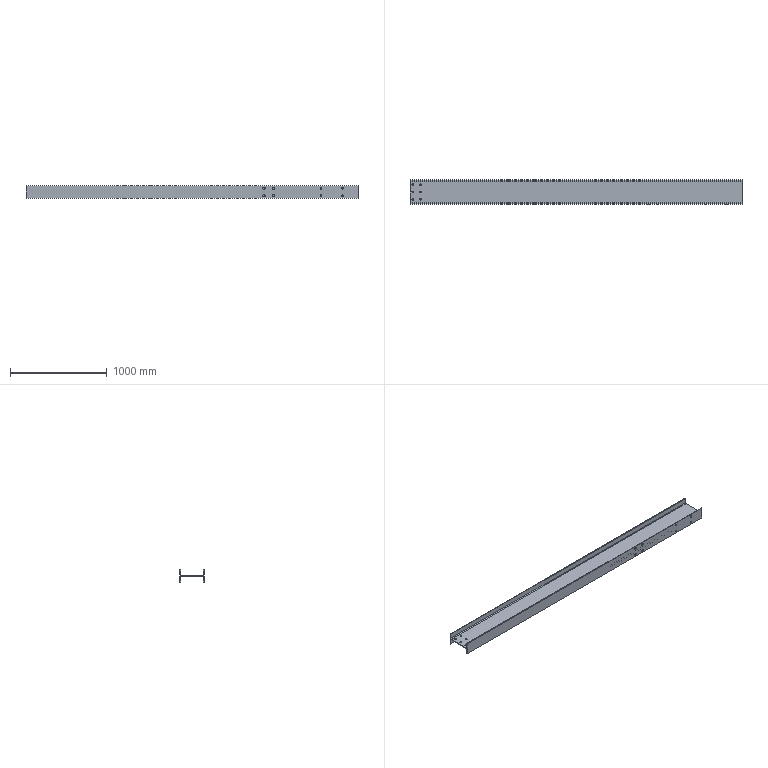Part | STEP file | Powder bin main beam 11 body_Default<As Machined> | 1 solid | 54 faces | box 3440 x 250 x 125 mm | volume 12683851 mm3 | cylinder 32 | plane 22 | commonest cylinder face diameters 19 x20 15 x8 16 x4